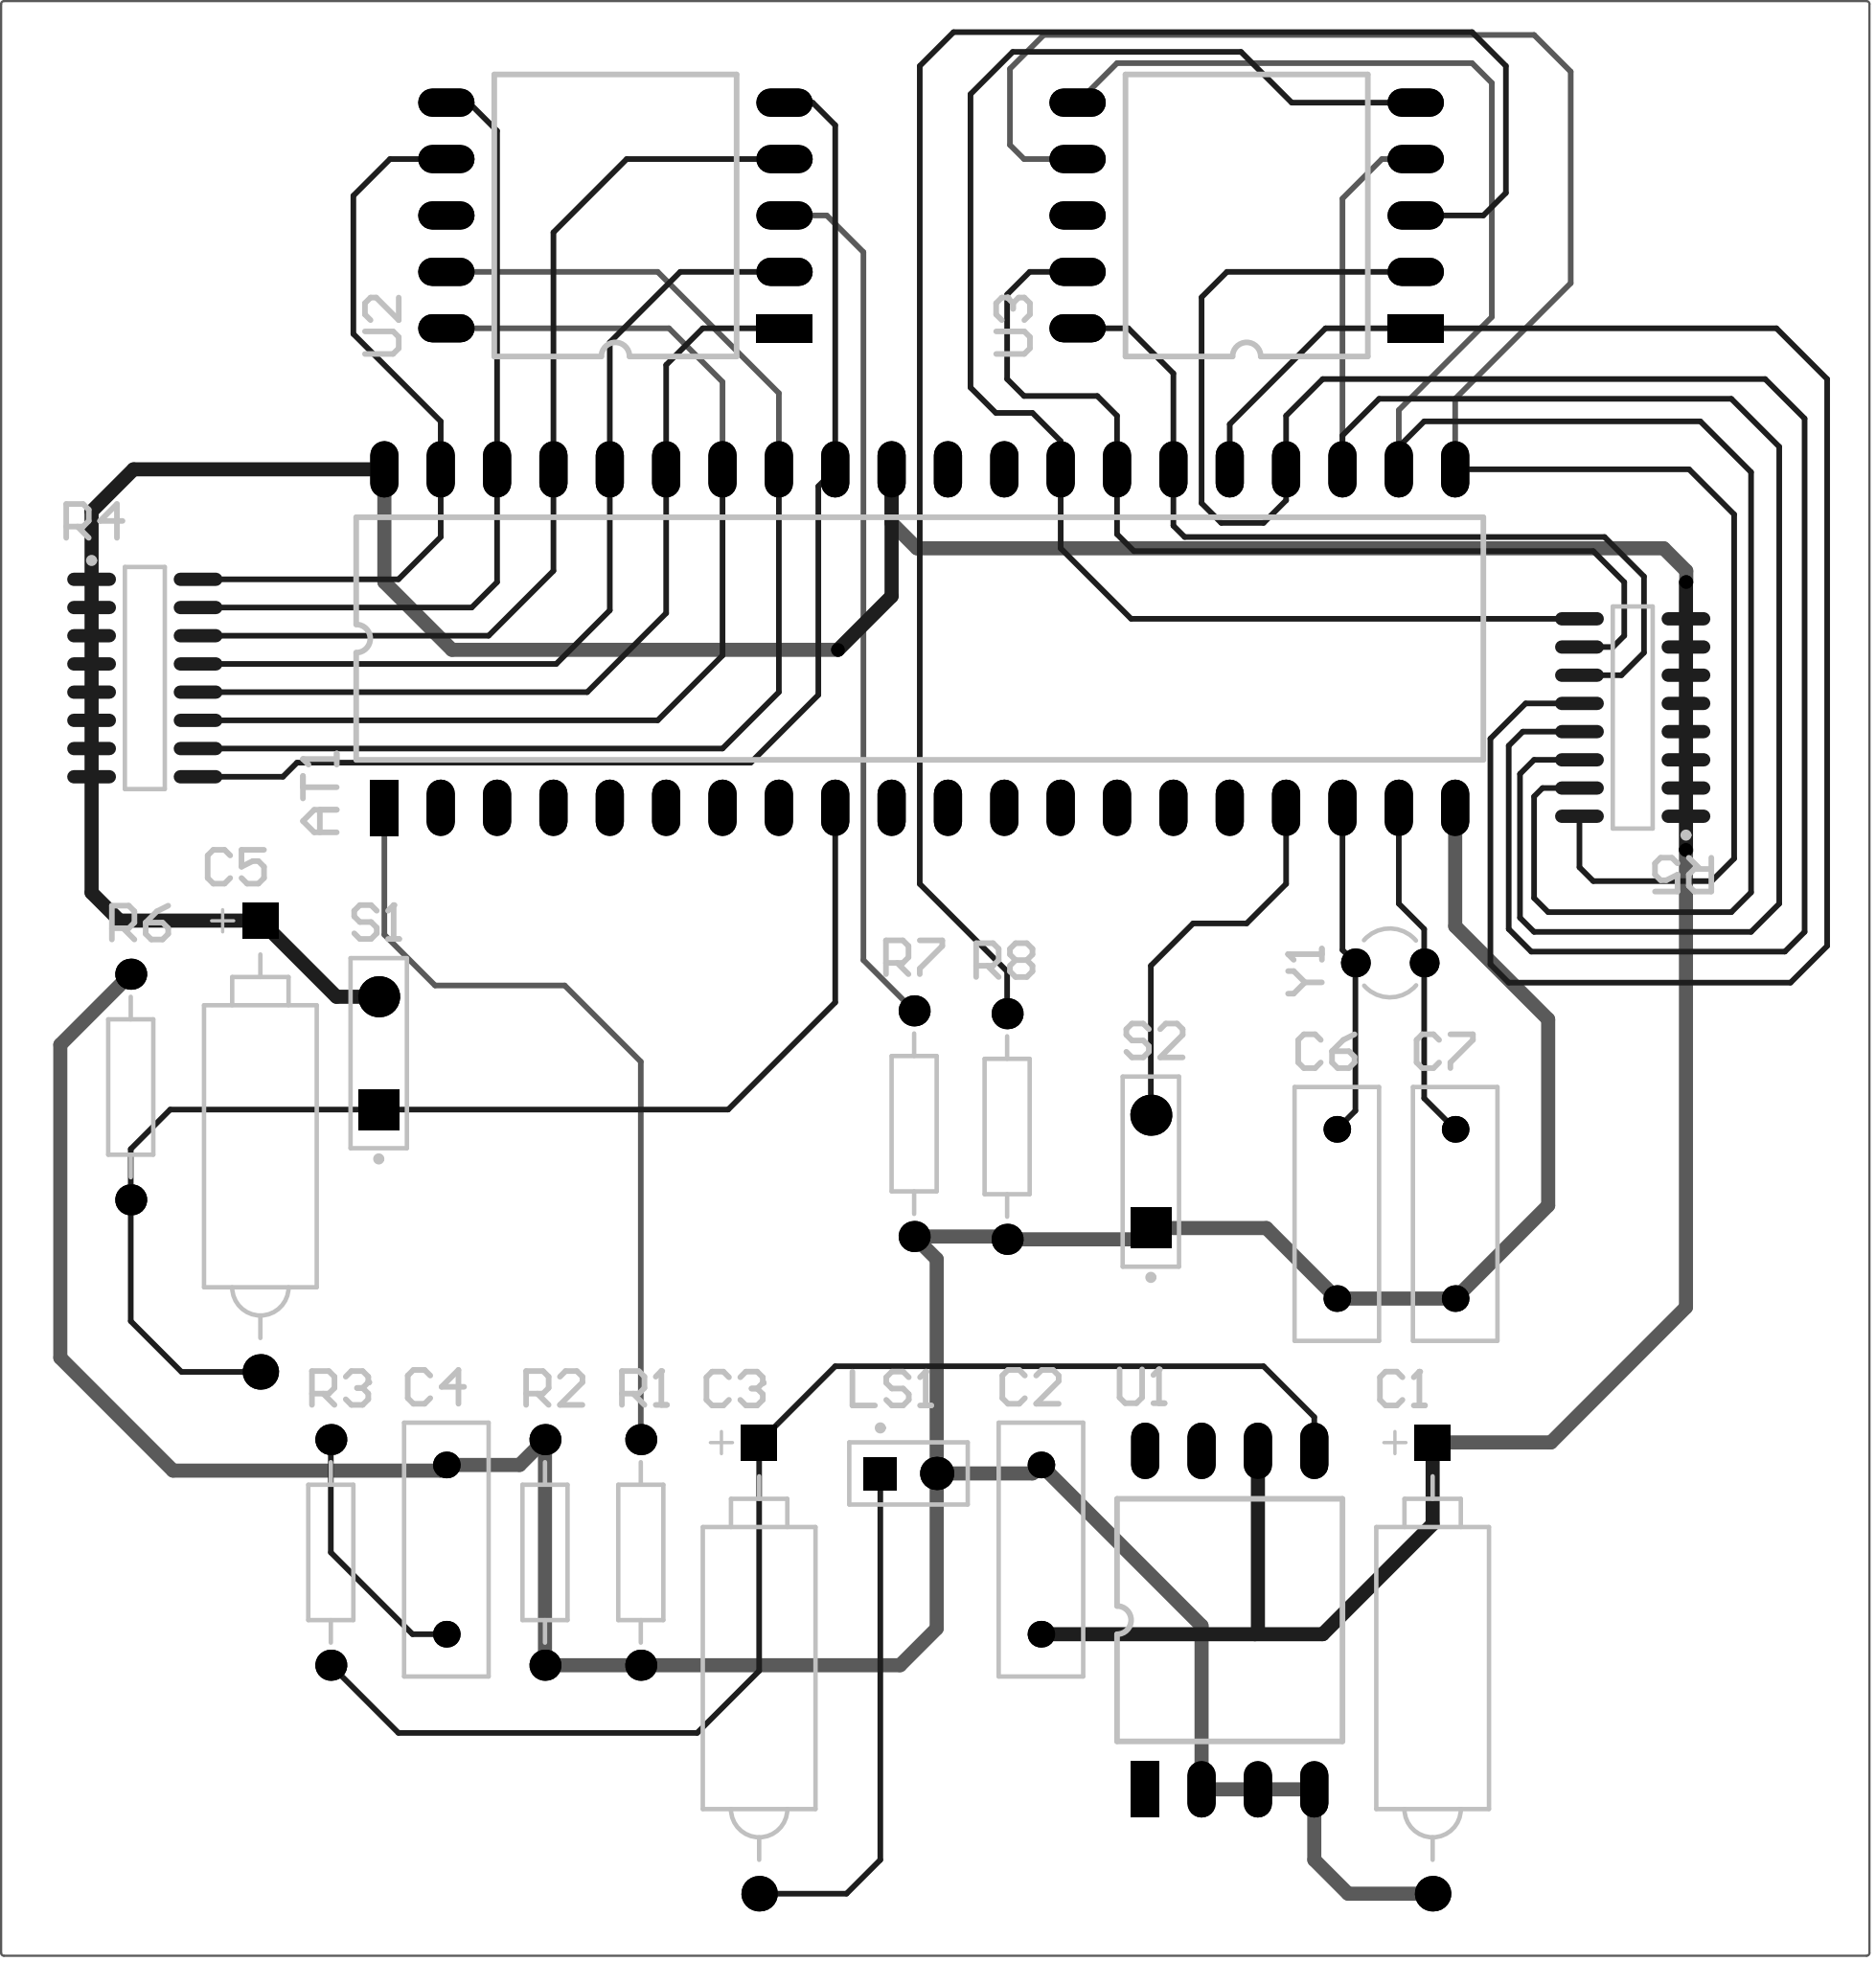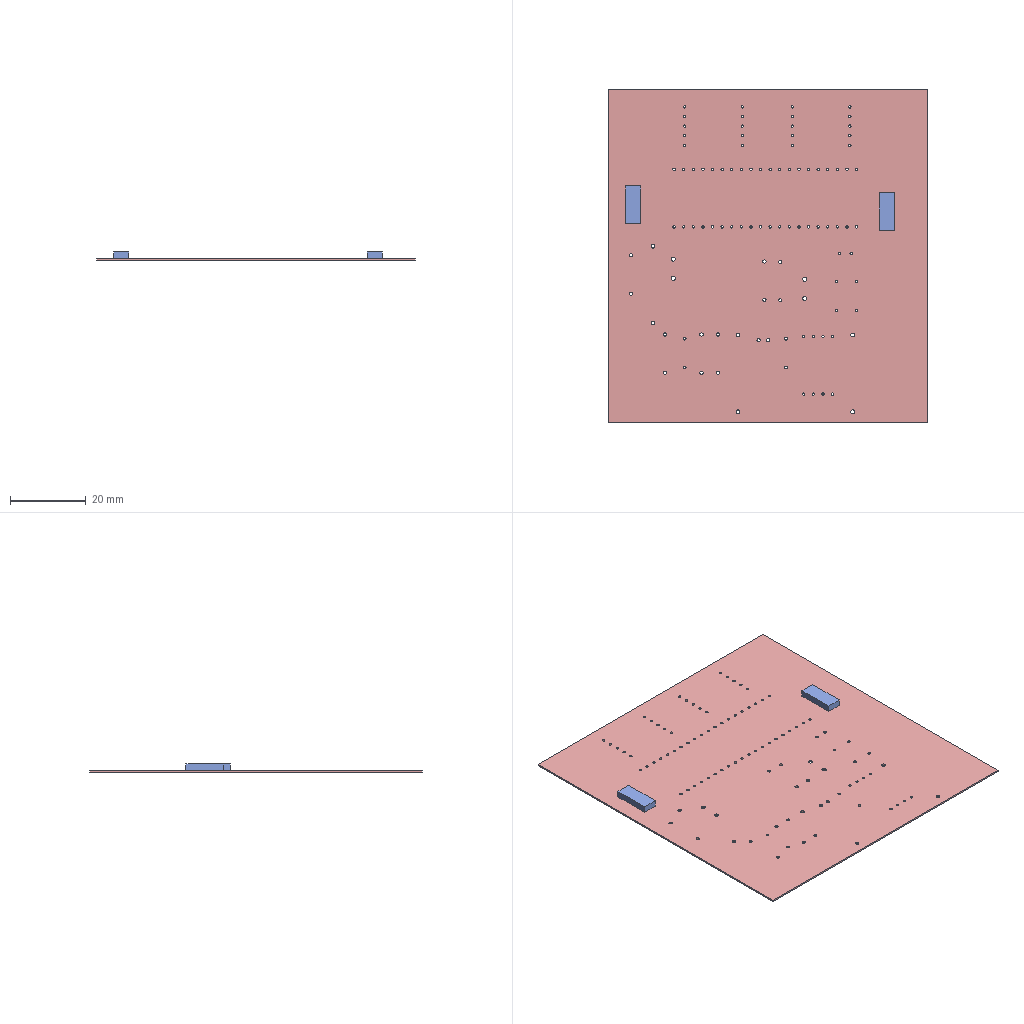Circuit board layout | Altium Designer | box 84.2 x 88 x 2.2 mm
Layer stack:
# Altium Designer layer stack of  (unit mm; dielectric type: 0 none, 1 core, 2 prepreg, 3 surface material)
index,name,kind,layer,copper_thickness_mm,dielectric_type,dielectric_thickness_mm,dielectric_material,dielectric_constant
0,Top Paste,other,,,,,,
1,Top Overlay,other,,,,,,
2,Top Solder,dielectric,,,3,0.0102,Solder Resist,3.5
3,Top Layer,copper,Top Layer,0.0356,,,,
4,Dielectric 1,dielectric,,,0,0.32,FR-4,4.8
5,Bottom Layer,copper,Bottom Layer,0.0356,,,,
6,Bottom Solder,dielectric,,,3,0.0102,Solder Resist,3.5
7,Bottom Overlay,other,,,,,,
8,Bottom Paste,other,,,,,,
# drill layer pairs: low layer,high layer
drill_pair,Top Layer,Bottom Layer
Part placement:
Designator,Comment,Layer,Footprint,Center-X(mm),Center-Y(mm),Rotation
Y1,XTAL,TopLayer,R38,102.336,69.977,90
U3,LED8,TopLayer,LED8,95.885,103.632,180
U2,LED8,TopLayer,LED8,67.437,103.632,180
U1,LM386N-1,TopLayer,LM386N-1,95.123,40.386,90
S2,SW-PB,TopLayer,SPST-2,91.567,60.579,90
S1,SW-PB,TopLayer,SPST-2,56.769,65.913,90
R8,10K,TopLayer,AXIAL-0.4,85.09,62.611,270
R7,10K,TopLayer,AXIAL-0.4,80.899,62.738,270
R6,10K,TopLayer,AXIAL-0.4,45.593,64.389,90
R5,Res Pack3,TopLayer,SO-16_N,113.284,81.026,180
R4,Res Pack3,TopLayer,SO-16_N,46.228,82.804,360
R3,47,TopLayer,AXIAL-0.4,54.61,43.434,90
R2,470,TopLayer,AXIAL-0.4,64.262,43.434,90
R1,10K,TopLayer,AXIAL-0.4,68.58,43.434,90
LS1,Speaker,TopLayer,PIN2,80.645,46.99,0
C7,30PF,TopLayer,RAD-0.3,105.283,58.674,90
C6,30PF,TopLayer,RAD-0.3,99.949,58.674,90
C5,10UF,TopLayer,POLAR0.8,51.435,61.722,90
C4,0.047UF,TopLayer,RAD-0.3,59.817,43.561,90
C3,47UF,TopLayer,POLAR0.8,73.914,38.227,90
C2,0.1UF,TopLayer,RAD-0.3,86.614,43.561,90
C1,10UF,TopLayer,POLAR0.8,104.267,38.227,90
AT1,U?,TopLayer,AT89S52,81.153,84.582,90
Pad and via stacks:
# Altium Designer via and pad stacks of  (unit mm). Each distinct definition once, with the count of objects using it.
# via: kind,start_layer,end_layer,hole_mm,diameter_mm,mode(0 simple;1 top-mid-bottom;2 full stack),diameter_per_layer,count,example_net
# pad: kind,layer,hole_mm,hole_type(0 round;1 square;2 slot),plating,top_size,top_shape(1 round;2 rect;3 octagon;9 rounded rect),mid_size,bottom_size,mode,footprint,size_per_layer,count,example
pad,Multi-Layer,1,0,plated,1.6x1.6,1,1.6x1.6,1.6x1.6,0,POLAR0.8,,3,C1.2
pad,Multi-Layer,1,0,plated,1.6x1.6,2,1.6x1.6,1.6x1.6,0,POLAR0.8,,3,C1.1
pad,Multi-Layer,0.635,0,plated,2.54x1.27,2,2.54x1.27,2.54x1.27,0,LM386N-1,,1,U1.1
pad,Multi-Layer,0.635,0,plated,2.54x1.27,1,2.54x1.27,2.54x1.27,0,LM386N-1,,7,U1.2
pad,Multi-Layer,0.7,0,plated,1.2x1.2,1,1.2x1.2,1.2x1.2,0,RAD-0.3,,8,C2.2
pad,Multi-Layer,0.9,0,plated,1.5x1.5,2,1.5x1.5,1.5x1.5,0,PIN2,,1,LS1.1
pad,Multi-Layer,0.9,0,plated,1.5x1.5,1,1.5x1.5,1.5x1.5,0,PIN2,,1,LS1.2
pad,Multi-Layer,0.85,0,plated,1.4x1.4,1,1.4x1.4,1.4x1.4,0,AXIAL-0.4,,12,R1.1
pad,Multi-Layer,1.1,0,plated,1.85x1.85,2,1.85x1.85,1.85x1.85,0,SPST-2,,2,S1.1
pad,Multi-Layer,1.1,0,plated,1.85x1.85,1,1.85x1.85,1.85x1.85,0,SPST-2,,2,S1.2
pad,Multi-Layer,0.635,0,plated,2.54x1.27,2,2.54x1.27,2.54x1.27,0,AT89S52,,1,AT1.1
pad,Multi-Layer,0.635,0,plated,2.54x1.27,1,2.54x1.27,2.54x1.27,0,AT89S52,,39,AT1.2
pad,Multi-Layer,0.635,0,plated,2.54x1.27,2,2.54x1.27,2.54x1.27,0,LED8,,2,U3.1
pad,Multi-Layer,0.635,0,plated,2.54x1.27,1,2.54x1.27,2.54x1.27,0,LED8,,18,U3.2
pad,Multi-Layer,0.7,0,plated,1.3x1.3,1,1.3x1.3,1.3x1.3,0,R38,,2,Y1.1
pad,Top Layer,0,0,plated,0.6x2.2,1,0.6x2.2,0.6x2.2,0,SO-16_N,,32,R5.1
via,Top Layer,Bottom Layer,0.3048,0.6096,0,,3,VCC
Design rules, without the lines most boards share:
# Altium Designer design rules of  (exported by Altium Designer, unit mm)
# columns: name | kind | enabled | priority | scope1 | scope2 | descriptor | typed fields (field=value)
SilkToSilkClearance | 55 | enabled | 1 | All | All | Silk to Silk (Clearance=0mil) (All),(All) |
SilkToSolderMaskClearance | 54 | enabled | 1 | IsPad | All | Silk To Solder Mask (Clearance=0mil) (IsPad),(All) |
MinimumSolderMaskSliver | 53 | enabled | 1 | All | All | Minimum Solder Mask Sliver (Gap=0mil) (All),(All) |
HoleToHoleClearance | 52 | enabled | 1 | All | All | Hole To Hole Clearance (Gap=10mil) (All),(All) | gap=0.254
DiffPairsRouting | 51 | enabled | 1 | All | All | Differential Pairs Uncoupled Length using the Gap Constraints (Min=10mil) (Max=10mil) (Prefered=10mil)  and Width Constraints (Min=15mil) (Max=15mil) (Prefered=15mil) (All) |
SolderMaskExpansion | 13 | enabled | 1 | All | All | Solder Mask Expansion (Expansion =4mil) (All) | expansion=0.1016
PasteMaskExpansion | 14 | enabled | 1 | All | All | Paste Mask Expansion (Expansion =0mil) (All) | expansion=0
RoutingVias | 11 | enabled | 1 | All | All | Routing Via (MinHoleWidth=28mil) (MaxHoleWidth=28mil) (PreferredHoleWidth=28mil) (MinWidth=50mil) (MaxWidth=50mil) (PreferedWidth=50mil) (All) | via_min_hole=0.7112 via_max_hole=0.7112 via_preferred_diameter=1.27 via_preferred_hole=0.7112
Width | 2 | enabled | 1 | All | All | Width Constraint (Min=10mil) (Max=30mil) (Preferred=10mil) (All) |
PolygonConnect | 20 | enabled | 1 | All | All | Polygon Connect Rule(Relief Connect )(Conductor Width=10mil) (Relief Angle=90 Angle) (Entries=4) (Air Gap Width=10mil) (All),(All) | connect_style(0=relief,1=direct,2=none)=0 relief_conductor_width=0.254 relief_entries=4
PlaneConnect | 6 | enabled | 1 | All | All | Power Plane Connect Rule(Relief Connect )(Expansion=20mil) (Conductor Width=10mil) (Air Gap=10mil) (Entries=4) (All) | relief_conductor_width=0.254 relief_entries=4 relief_expansion=0.508
Clearance | 0 | enabled | 1 | All | All | Clearance Constraint (Gap=10mil) (All),(All) | gap=0.254
Classes set for this board:
# Altium Designer classes of  (member kind: 0 net, 1 component, 2 from-to, 3 pad, 4 layer, 5 differential pair, 6 design channel, 7 polygon, 8 structure, 9 xSignal)
# columns: class name | member kind | superclass | members
Sheet1 | 1 | no | AT1; C1; C2; C3; C4; C5; C6; C7; LS1; R1; R2; R3; R4; R5; R6; R7; R8; S1; S2; U1; U2; U3; Y1;